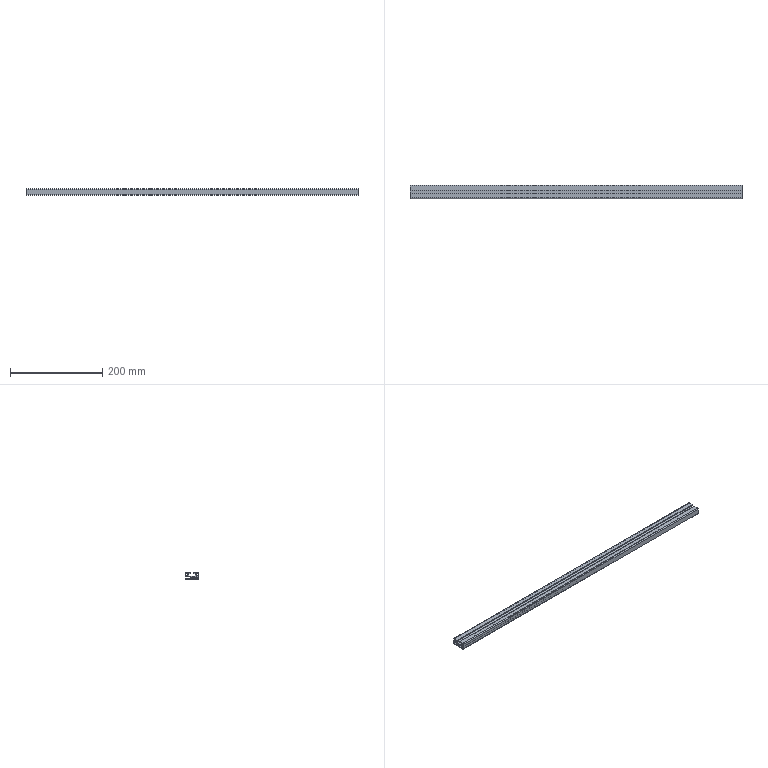Part | STEP file | 01.1.015030-L-00 magazine hanger profile 15x30-1269 | 1 solid | 38 faces | box 720 x 30 x 15 mm | volume 154915 mm3 | plane 30 | cylinder 8 | commonest cylinder face diameters 4 x4 4.5 x4